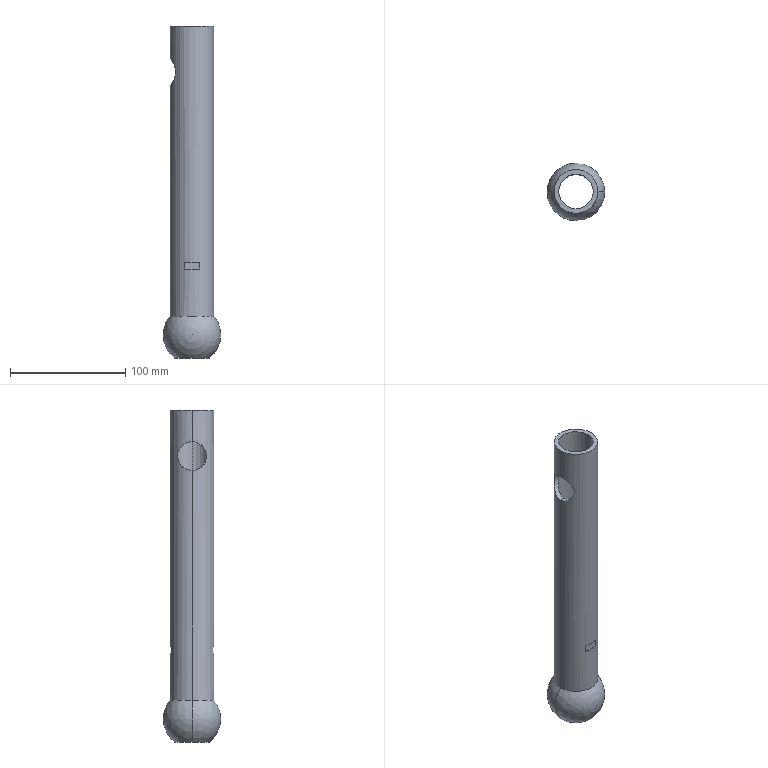Part | STEP file | Feed pipe SGN-6-02 | 1 solid | 15 faces | box 50 x 50 x 288.248 mm | volume 138112 mm3 | plane 7 | cylinder 6 | sphere 2 | commonest cylinder face diameters 25 x2 30 x2 38 x2